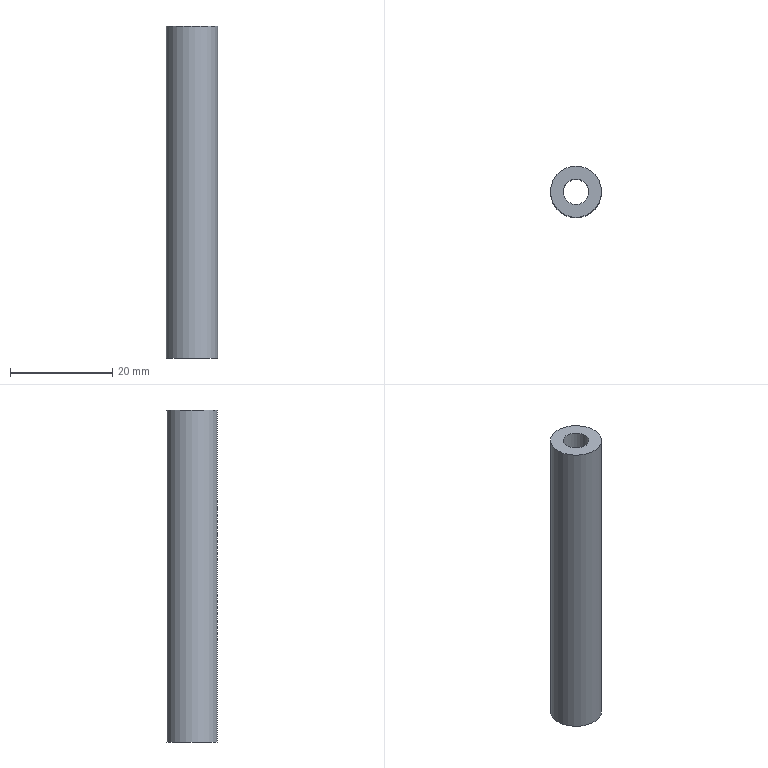Part | NX | features DATUM_CSYS 1, EXTRACT_DATUM_PLANE 1, EXTRUDE 1, SKETCH 1 | 1 solid | 4 faces | box 10 x 10 x 65 mm | volume 3829 mm3 | cylinder 2 | plane 2 | commonest cylinder face diameters 5 x1 10 x1
STEP:
#1=CARTESIAN_POINT('',(5.,0.,-32.5));
#2=VERTEX_POINT('',#1);
#3=CARTESIAN_POINT('',(0.,0.,-32.5));
#4=DIRECTION('',(0.,0.,1.));
#5=DIRECTION('',(1.,0.,0.));
#6=AXIS2_PLACEMENT_3D('',#3,#4,#5);
#7=CIRCLE('',#6,5.);
#8=EDGE_CURVE('',#2,#2,#7,.T.);
#9=ORIENTED_EDGE('',*,*,#8,.T.);
#10=EDGE_LOOP('',(#9));
#11=FACE_BOUND('',#10,.T.);
#12=CARTESIAN_POINT('',(-5.,0.,32.5));
#13=VERTEX_POINT('',#12);
#14=CARTESIAN_POINT('',(0.,0.,32.5));
#15=DIRECTION('',(0.,0.,1.));
#16=DIRECTION('',(-1.,0.,0.));
#17=AXIS2_PLACEMENT_3D('',#14,#15,#16);
#18=CIRCLE('',#17,5.);
#19=EDGE_CURVE('',#13,#13,#18,.T.);
#20=ORIENTED_EDGE('',*,*,#19,.F.);
#21=EDGE_LOOP('',(#20));
#22=FACE_BOUND('',#21,.T.);
#23=CARTESIAN_POINT('',(0.,0.,32.5));
#24=DIRECTION('',(0.,0.,-1.));
#25=DIRECTION('',(-1.,0.,0.));
#26=AXIS2_PLACEMENT_3D('',#23,#24,#25);
#27=CYLINDRICAL_SURFACE('',#26,5.);
#28=ADVANCED_FACE('',(#11,#22),#27,.T.);
#29=CARTESIAN_POINT('',(-2.5,0.,-32.5));
#30=VERTEX_POINT('',#29);
#31=CARTESIAN_POINT('',(0.,0.,-32.5));
#32=DIRECTION('',(0.,0.,1.));
#33=DIRECTION('',(-1.,0.,0.));
#34=AXIS2_PLACEMENT_3D('',#31,#32,#33);
#35=CIRCLE('',#34,2.5);
#36=EDGE_CURVE('',#30,#30,#35,.T.);
#37=ORIENTED_EDGE('',*,*,#36,.F.);
#38=EDGE_LOOP('',(#37));
#39=FACE_BOUND('',#38,.T.);
#40=CARTESIAN_POINT('',(2.5,0.,32.5));
#41=VERTEX_POINT('',#40);
#42=CARTESIAN_POINT('',(0.,0.,32.5));
#43=DIRECTION('',(0.,0.,1.));
#44=DIRECTION('',(1.,0.,0.));
#45=AXIS2_PLACEMENT_3D('',#42,#43,#44);
#46=CIRCLE('',#45,2.5);
#47=EDGE_CURVE('',#41,#41,#46,.T.);
#48=ORIENTED_EDGE('',*,*,#47,.T.);
#49=EDGE_LOOP('',(#48));
#50=FACE_BOUND('',#49,.T.);
#51=CARTESIAN_POINT('',(0.,0.,32.5));
#52=DIRECTION('',(0.,0.,-1.));
#53=DIRECTION('',(-1.,0.,0.));
#54=AXIS2_PLACEMENT_3D('',#51,#52,#53);
#55=CYLINDRICAL_SURFACE('',#54,2.5);
#56=ADVANCED_FACE('',(#39,#50),#55,.F.);
#57=ORIENTED_EDGE('',*,*,#19,.T.);
#58=EDGE_LOOP('',(#57));
#59=FACE_BOUND('',#58,.T.);
#60=ORIENTED_EDGE('',*,*,#47,.F.);
#61=EDGE_LOOP('',(#60));
#62=FACE_BOUND('',#61,.T.);
#63=CARTESIAN_POINT('',(0.,0.,32.5));
#64=DIRECTION('',(0.,0.,1.));
#65=DIRECTION('',(1.,0.,0.));
#66=AXIS2_PLACEMENT_3D('',#63,#64,#65);
#67=PLANE('',#66);
#68=ADVANCED_FACE('',(#59,#62),#67,.T.);
#69=ORIENTED_EDGE('',*,*,#8,.F.);
#70=EDGE_LOOP('',(#69));
#71=FACE_BOUND('',#70,.T.);
#72=ORIENTED_EDGE('',*,*,#36,.T.);
#73=EDGE_LOOP('',(#72));
#74=FACE_BOUND('',#73,.T.);
#75=CARTESIAN_POINT('',(0.,0.,-32.5));
#76=DIRECTION('',(0.,0.,1.));
#77=DIRECTION('',(1.,0.,0.));
#78=AXIS2_PLACEMENT_3D('',#75,#76,#77);
#79=PLANE('',#78);
#80=ADVANCED_FACE('',(#71,#74),#79,.F.);
#81=CLOSED_SHELL('',(#28,#56,#68,#80));
#82=MANIFOLD_SOLID_BREP('',#81);
#83=(LENGTH_UNIT()NAMED_UNIT(*)SI_UNIT(.MILLI.,.METRE.));
#84=UNCERTAINTY_MEASURE_WITH_UNIT(LENGTH_MEASURE(0.00001),#83,'','');
#85=(NAMED_UNIT(*)PLANE_ANGLE_UNIT()SI_UNIT($,.RADIAN.));
#86=(NAMED_UNIT(*)SI_UNIT($,.STERADIAN.)SOLID_ANGLE_UNIT());
#87=(GEOMETRIC_REPRESENTATION_CONTEXT(3)GLOBAL_UNCERTAINTY_ASSIGNED_CONTEXT((#84))GLOBAL_UNIT_ASSIGNED_CONTEXT((#83,#85,#86))REPRESENTATION_CONTEXT('',''));
#88=ADVANCED_BREP_SHAPE_REPRESENTATION('',(#82),#87);